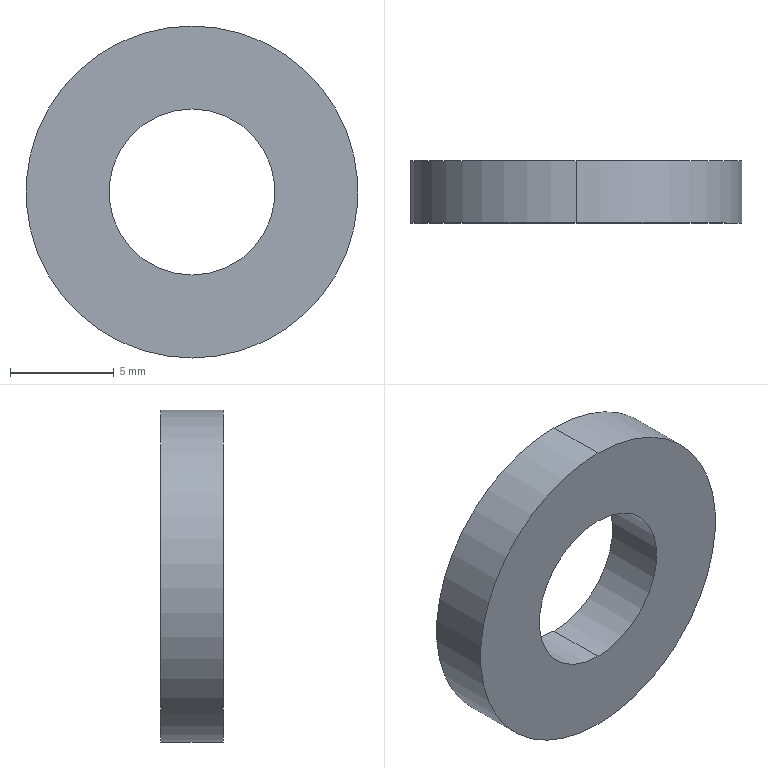Part | SolidWorks | features Extrusion 1 | 1 solid | 6 faces | box 16 x 3 x 16 mm | volume 452.389 mm3 | cylinder 4 | plane 2 | commonest cylinder face diameters 8 x2 16 x2
STEP:
#1=CARTESIAN_POINT('',(0.,3.,-4.));
#2=VERTEX_POINT('',#1);
#3=CARTESIAN_POINT('',(0.,3.,4.));
#4=VERTEX_POINT('',#3);
#5=CARTESIAN_POINT('',(0.,3.,0.));
#6=DIRECTION('',(0.,1.,0.));
#7=DIRECTION('',(0.,0.,1.));
#8=AXIS2_PLACEMENT_3D('',#5,#6,#7);
#9=CIRCLE('',#8,4.);
#10=EDGE_CURVE('',#2,#4,#9,.T.);
#11=ORIENTED_EDGE('',*,*,#10,.T.);
#12=CARTESIAN_POINT('',(0.,0.,4.));
#13=VERTEX_POINT('',#12);
#14=CARTESIAN_POINT('',(0.,3.,4.));
#15=DIRECTION('',(0.,-1.,0.));
#16=VECTOR('',#15,1000.);
#17=LINE('',#14,#16);
#18=EDGE_CURVE('',#4,#13,#17,.T.);
#19=ORIENTED_EDGE('',*,*,#18,.T.);
#20=CARTESIAN_POINT('',(0.,0.,-4.));
#21=VERTEX_POINT('',#20);
#22=CARTESIAN_POINT('',(0.,0.,0.));
#23=DIRECTION('',(0.,1.,0.));
#24=DIRECTION('',(0.,0.,1.));
#25=AXIS2_PLACEMENT_3D('',#22,#23,#24);
#26=CIRCLE('',#25,4.);
#27=EDGE_CURVE('',#21,#13,#26,.T.);
#28=ORIENTED_EDGE('',*,*,#27,.F.);
#29=CARTESIAN_POINT('',(0.,3.,-4.));
#30=DIRECTION('',(0.,-1.,0.));
#31=VECTOR('',#30,1000.);
#32=LINE('',#29,#31);
#33=EDGE_CURVE('',#2,#21,#32,.T.);
#34=ORIENTED_EDGE('',*,*,#33,.F.);
#35=EDGE_LOOP('',(#11,#19,#28,#34));
#36=FACE_OUTER_BOUND('',#35,.T.);
#37=CARTESIAN_POINT('',(0.,3.,0.));
#38=DIRECTION('',(0.,-1.,0.));
#39=DIRECTION('',(0.,0.,-1.));
#40=AXIS2_PLACEMENT_3D('',#37,#38,#39);
#41=CYLINDRICAL_SURFACE('',#40,4.);
#42=ADVANCED_FACE('',(#36),#41,.F.);
#43=CARTESIAN_POINT('',(0.,3.,8.));
#44=VERTEX_POINT('',#43);
#45=CARTESIAN_POINT('',(0.,3.,-8.));
#46=VERTEX_POINT('',#45);
#47=CARTESIAN_POINT('',(0.,3.,0.));
#48=DIRECTION('',(0.,1.,0.));
#49=DIRECTION('',(0.,0.,1.));
#50=AXIS2_PLACEMENT_3D('',#47,#48,#49);
#51=CIRCLE('',#50,8.);
#52=EDGE_CURVE('',#44,#46,#51,.T.);
#53=ORIENTED_EDGE('',*,*,#52,.F.);
#54=CARTESIAN_POINT('',(0.,0.,8.));
#55=VERTEX_POINT('',#54);
#56=CARTESIAN_POINT('',(0.,3.,8.));
#57=DIRECTION('',(0.,-1.,0.));
#58=VECTOR('',#57,1000.);
#59=LINE('',#56,#58);
#60=EDGE_CURVE('',#44,#55,#59,.T.);
#61=ORIENTED_EDGE('',*,*,#60,.T.);
#62=CARTESIAN_POINT('',(0.,0.,-8.));
#63=VERTEX_POINT('',#62);
#64=CARTESIAN_POINT('',(0.,0.,0.));
#65=DIRECTION('',(0.,1.,0.));
#66=DIRECTION('',(0.,0.,1.));
#67=AXIS2_PLACEMENT_3D('',#64,#65,#66);
#68=CIRCLE('',#67,8.);
#69=EDGE_CURVE('',#55,#63,#68,.T.);
#70=ORIENTED_EDGE('',*,*,#69,.T.);
#71=CARTESIAN_POINT('',(0.,3.,-8.));
#72=DIRECTION('',(0.,-1.,0.));
#73=VECTOR('',#72,1000.);
#74=LINE('',#71,#73);
#75=EDGE_CURVE('',#46,#63,#74,.T.);
#76=ORIENTED_EDGE('',*,*,#75,.F.);
#77=EDGE_LOOP('',(#53,#61,#70,#76));
#78=FACE_OUTER_BOUND('',#77,.T.);
#79=CARTESIAN_POINT('',(0.,3.,0.));
#80=DIRECTION('',(0.,-1.,0.));
#81=DIRECTION('',(0.,0.,-1.));
#82=AXIS2_PLACEMENT_3D('',#79,#80,#81);
#83=CYLINDRICAL_SURFACE('',#82,8.);
#84=ADVANCED_FACE('',(#78),#83,.T.);
#85=CARTESIAN_POINT('',(0.,3.,0.));
#86=DIRECTION('',(0.,1.,0.));
#87=DIRECTION('',(0.,0.,1.));
#88=AXIS2_PLACEMENT_3D('',#85,#86,#87);
#89=CIRCLE('',#88,8.);
#90=EDGE_CURVE('',#46,#44,#89,.T.);
#91=ORIENTED_EDGE('',*,*,#90,.T.);
#92=ORIENTED_EDGE('',*,*,#52,.T.);
#93=EDGE_LOOP('',(#91,#92));
#94=FACE_OUTER_BOUND('',#93,.T.);
#95=ORIENTED_EDGE('',*,*,#10,.F.);
#96=CARTESIAN_POINT('',(0.,3.,0.));
#97=DIRECTION('',(0.,1.,0.));
#98=DIRECTION('',(0.,0.,1.));
#99=AXIS2_PLACEMENT_3D('',#96,#97,#98);
#100=CIRCLE('',#99,4.);
#101=EDGE_CURVE('',#4,#2,#100,.T.);
#102=ORIENTED_EDGE('',*,*,#101,.F.);
#103=EDGE_LOOP('',(#95,#102));
#104=FACE_BOUND('',#103,.T.);
#105=CARTESIAN_POINT('',(0.,3.,0.));
#106=DIRECTION('',(0.,1.,0.));
#107=DIRECTION('',(0.,0.,1.));
#108=AXIS2_PLACEMENT_3D('',#105,#106,#107);
#109=PLANE('',#108);
#110=ADVANCED_FACE('',(#94,#104),#109,.T.);
#111=CARTESIAN_POINT('',(0.,0.,0.));
#112=DIRECTION('',(0.,1.,0.));
#113=DIRECTION('',(0.,0.,1.));
#114=AXIS2_PLACEMENT_3D('',#111,#112,#113);
#115=CIRCLE('',#114,8.);
#116=EDGE_CURVE('',#63,#55,#115,.T.);
#117=ORIENTED_EDGE('',*,*,#116,.F.);
#118=ORIENTED_EDGE('',*,*,#69,.F.);
#119=EDGE_LOOP('',(#117,#118));
#120=FACE_OUTER_BOUND('',#119,.T.);
#121=ORIENTED_EDGE('',*,*,#27,.T.);
#122=CARTESIAN_POINT('',(0.,0.,0.));
#123=DIRECTION('',(0.,1.,0.));
#124=DIRECTION('',(0.,0.,1.));
#125=AXIS2_PLACEMENT_3D('',#122,#123,#124);
#126=CIRCLE('',#125,4.);
#127=EDGE_CURVE('',#13,#21,#126,.T.);
#128=ORIENTED_EDGE('',*,*,#127,.T.);
#129=EDGE_LOOP('',(#121,#128));
#130=FACE_BOUND('',#129,.T.);
#131=CARTESIAN_POINT('',(0.,0.,0.));
#132=DIRECTION('',(0.,1.,0.));
#133=DIRECTION('',(0.,0.,1.));
#134=AXIS2_PLACEMENT_3D('',#131,#132,#133);
#135=PLANE('',#134);
#136=ADVANCED_FACE('',(#120,#130),#135,.F.);
#137=ORIENTED_EDGE('',*,*,#60,.F.);
#138=ORIENTED_EDGE('',*,*,#90,.F.);
#139=ORIENTED_EDGE('',*,*,#75,.T.);
#140=ORIENTED_EDGE('',*,*,#116,.T.);
#141=EDGE_LOOP('',(#137,#138,#139,#140));
#142=FACE_OUTER_BOUND('',#141,.T.);
#143=CARTESIAN_POINT('',(0.,3.,0.));
#144=DIRECTION('',(0.,-1.,0.));
#145=DIRECTION('',(0.,0.,-1.));
#146=AXIS2_PLACEMENT_3D('',#143,#144,#145);
#147=CYLINDRICAL_SURFACE('',#146,8.);
#148=ADVANCED_FACE('',(#142),#147,.T.);
#149=ORIENTED_EDGE('',*,*,#18,.F.);
#150=ORIENTED_EDGE('',*,*,#101,.T.);
#151=ORIENTED_EDGE('',*,*,#33,.T.);
#152=ORIENTED_EDGE('',*,*,#127,.F.);
#153=EDGE_LOOP('',(#149,#150,#151,#152));
#154=FACE_OUTER_BOUND('',#153,.T.);
#155=CARTESIAN_POINT('',(0.,3.,0.));
#156=DIRECTION('',(0.,-1.,0.));
#157=DIRECTION('',(0.,0.,-1.));
#158=AXIS2_PLACEMENT_3D('',#155,#156,#157);
#159=CYLINDRICAL_SURFACE('',#158,4.);
#160=ADVANCED_FACE('',(#154),#159,.F.);
#161=CLOSED_SHELL('',(#42,#84,#110,#136,#148,#160));
#162=MANIFOLD_SOLID_BREP('',#161);
#163=CARTESIAN_POINT('',(0.,0.,0.));
#164=DIRECTION('',(0.,0.,1.));
#165=DIRECTION('',(1.,0.,0.));
#166=AXIS2_PLACEMENT_3D('',#163,#164,#165);
#167=(LENGTH_UNIT()NAMED_UNIT(*)SI_UNIT(.MILLI.,.METRE.));
#168=UNCERTAINTY_MEASURE_WITH_UNIT(LENGTH_MEASURE(0.00001),#167,'','');
#169=(NAMED_UNIT(*)PLANE_ANGLE_UNIT()SI_UNIT($,.RADIAN.));
#170=(NAMED_UNIT(*)SI_UNIT($,.STERADIAN.)SOLID_ANGLE_UNIT());
#171=(GEOMETRIC_REPRESENTATION_CONTEXT(3)GLOBAL_UNCERTAINTY_ASSIGNED_CONTEXT((#168))GLOBAL_UNIT_ASSIGNED_CONTEXT((#167,#169,#170))REPRESENTATION_CONTEXT('',''));
#172=ADVANCED_BREP_SHAPE_REPRESENTATION('',(#162,#166),#171);